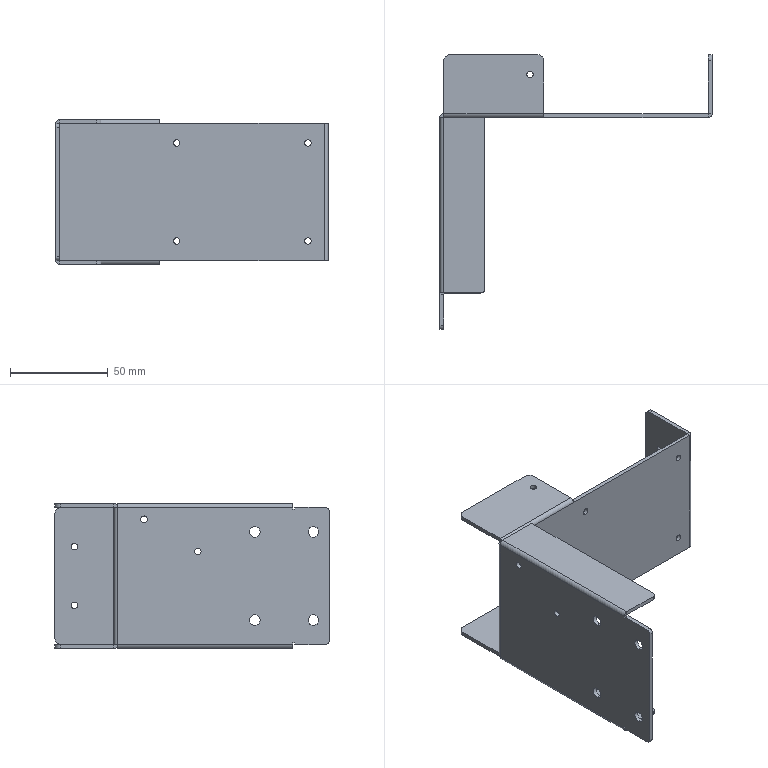Part | STEP file | 1 solid | 104 faces | box 139.01 x 140 x 74.02 mm | volume 52784 mm3 | plane 54 | cylinder 50 | commonest cylinder face diameters 3.3 x20 5.5 x8 0.02 x6 4.02 x6 6 x6 4 x4